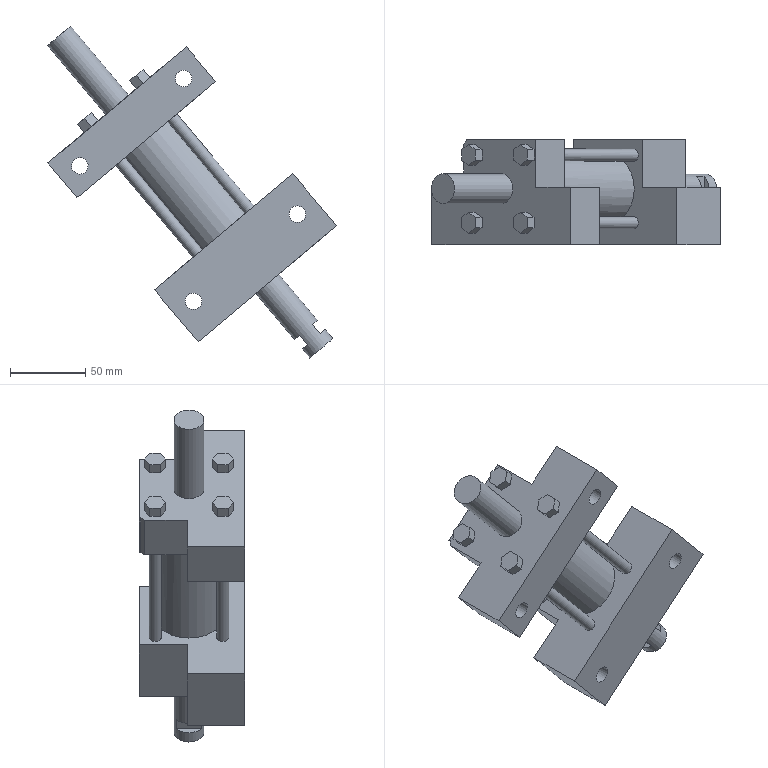Part | STEP file | solid 153 | 1 solid | 81 faces | box 191.822 x 70 x 220.454 mm | volume 648426 mm3 | plane 62 | cylinder 17 | cone 2 | commonest cylinder face diameters 8 x4 11 x4 18 x4 15 x2 20 x2 46 x1